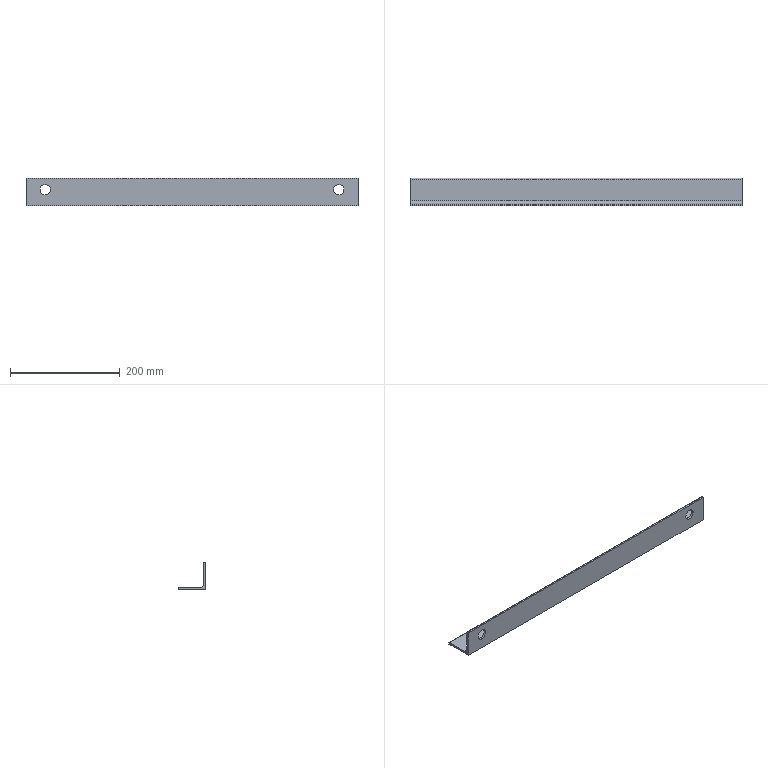Part | STEP file | 计量角钢1_Default<As Machined> | 1 solid | 15 faces | box 605 x 50 x 50 mm | volume 233520 mm3 | plane 8 | cylinder 7 | commonest cylinder face diameters 19 x4 2.66 x2 11 x1
STEP:
#1=CARTESIAN_POINT('',(0.,0.,0.));
#2=DIRECTION('',(0.,0.,1.));
#3=DIRECTION('',(1.,0.,0.));
#4=AXIS2_PLACEMENT_3D('',#1,#2,#3);
#5=CARTESIAN_POINT('',(-267.5,0.,38.585));
#6=VERTEX_POINT('',#5);
#7=CARTESIAN_POINT('',(-267.5,4.,38.585));
#8=VERTEX_POINT('',#7);
#9=CARTESIAN_POINT('',(-267.5,-6.,38.585));
#10=DIRECTION('',(0.,1.,0.));
#11=VECTOR('',#10,1.);
#12=LINE('',#9,#11);
#13=CARTESIAN_POINT('',(-267.5,-6.,29.085));
#14=DIRECTION('',(0.,1.,0.));
#15=DIRECTION('',(0.,0.,1.));
#16=AXIS2_PLACEMENT_3D('',#13,#14,#15);
#17=CYLINDRICAL_SURFACE('',#16,9.5);
#18=CARTESIAN_POINT('',(6.283,0.));
#19=DIRECTION('',(0.,1.));
#20=VECTOR('',#19,1.);
#21=LINE('',#18,#20);
#22=(GEOMETRIC_REPRESENTATION_CONTEXT(2)PARAMETRIC_REPRESENTATION_CONTEXT()REPRESENTATION_CONTEXT('',''));
#23=DEFINITIONAL_REPRESENTATION('',(#21),#22);
#24=PCURVE('',#17,#23);
#25=CARTESIAN_POINT('',(-267.5,-6.,29.085));
#26=DIRECTION('',(0.,1.,0.));
#27=DIRECTION('',(0.,0.,1.));
#28=AXIS2_PLACEMENT_3D('',#25,#26,#27);
#29=CYLINDRICAL_SURFACE('',#28,9.5);
#30=CARTESIAN_POINT('',(0.,0.));
#31=DIRECTION('',(0.,1.));
#32=VECTOR('',#31,1.);
#33=LINE('',#30,#32);
#34=(GEOMETRIC_REPRESENTATION_CONTEXT(2)PARAMETRIC_REPRESENTATION_CONTEXT()REPRESENTATION_CONTEXT('',''));
#35=DEFINITIONAL_REPRESENTATION('',(#33),#34);
#36=PCURVE('',#29,#35);
#37=SURFACE_CURVE('',#12,(#24,#36),.PCURVE_S1.);
#38=EDGE_CURVE('',#6,#8,#37,.T.);
#39=ORIENTED_EDGE('',*,*,#38,.T.);
#40=CARTESIAN_POINT('',(-267.5,4.,19.585));
#41=VERTEX_POINT('',#40);
#42=CARTESIAN_POINT('',(-267.5,4.,29.085));
#43=DIRECTION('',(0.,1.,0.));
#44=DIRECTION('',(0.,0.,1.));
#45=AXIS2_PLACEMENT_3D('',#42,#43,#44);
#46=CIRCLE('',#45,9.5);
#47=CARTESIAN_POINT('',(0.,10.));
#48=DIRECTION('',(1.,0.));
#49=VECTOR('',#48,1.);
#50=LINE('',#47,#49);
#51=(GEOMETRIC_REPRESENTATION_CONTEXT(2)PARAMETRIC_REPRESENTATION_CONTEXT()REPRESENTATION_CONTEXT('',''));
#52=DEFINITIONAL_REPRESENTATION('',(#50),#51);
#53=PCURVE('',#17,#52);
#54=CARTESIAN_POINT('',(302.5,4.,48.67));
#55=DIRECTION('',(0.,-1.,0.));
#56=DIRECTION('',(1.,0.,0.));
#57=AXIS2_PLACEMENT_3D('',#54,#55,#56);
#58=PLANE('',#57);
#59=CARTESIAN_POINT('',(-570.,-10.085));
#60=CARTESIAN_POINT('',(-553.546,-10.085));
#61=CARTESIAN_POINT('',(-561.773,-24.335));
#62=CARTESIAN_POINT('',(-570.,-38.585));
#63=CARTESIAN_POINT('',(-578.227,-24.335));
#64=CARTESIAN_POINT('',(-586.454,-10.085));
#65=CARTESIAN_POINT('',(-570.,-10.085));
#66=(BOUNDED_CURVE()B_SPLINE_CURVE(2,(#59,#60,#61,#62,#63,#64,#65),.UNSPECIFIED.,.T.,.F.)B_SPLINE_CURVE_WITH_KNOTS((1,2,2,2,2,1),(-2.094,0.,2.094,4.189,6.283,8.378),.UNSPECIFIED.)CURVE()GEOMETRIC_REPRESENTATION_ITEM()RATIONAL_B_SPLINE_CURVE((1.,0.5,1.,0.5,1.,0.5,1.))REPRESENTATION_ITEM(''));
#67=(GEOMETRIC_REPRESENTATION_CONTEXT(2)PARAMETRIC_REPRESENTATION_CONTEXT()REPRESENTATION_CONTEXT('',''));
#68=DEFINITIONAL_REPRESENTATION('',(#66),#67);
#69=PCURVE('',#58,#68);
#70=SURFACE_CURVE('',#46,(#53,#69),.PCURVE_S1.);
#71=EDGE_CURVE('',#41,#8,#70,.T.);
#72=ORIENTED_EDGE('',*,*,#71,.F.);
#73=CARTESIAN_POINT('',(-267.5,0.,19.585));
#74=VERTEX_POINT('',#73);
#75=CARTESIAN_POINT('',(-267.5,-6.,19.585));
#76=DIRECTION('',(0.,1.,0.));
#77=VECTOR('',#76,1.);
#78=LINE('',#75,#77);
#79=CARTESIAN_POINT('',(3.142,0.));
#80=DIRECTION('',(0.,1.));
#81=VECTOR('',#80,1.);
#82=LINE('',#79,#81);
#83=(GEOMETRIC_REPRESENTATION_CONTEXT(2)PARAMETRIC_REPRESENTATION_CONTEXT()REPRESENTATION_CONTEXT('',''));
#84=DEFINITIONAL_REPRESENTATION('',(#82),#83);
#85=PCURVE('',#17,#84);
#86=CARTESIAN_POINT('',(3.142,0.));
#87=DIRECTION('',(0.,1.));
#88=VECTOR('',#87,1.);
#89=LINE('',#86,#88);
#90=(GEOMETRIC_REPRESENTATION_CONTEXT(2)PARAMETRIC_REPRESENTATION_CONTEXT()REPRESENTATION_CONTEXT('',''));
#91=DEFINITIONAL_REPRESENTATION('',(#89),#90);
#92=PCURVE('',#29,#91);
#93=SURFACE_CURVE('',#78,(#85,#92),.PCURVE_S1.);
#94=EDGE_CURVE('',#74,#41,#93,.T.);
#95=ORIENTED_EDGE('',*,*,#94,.F.);
#96=CARTESIAN_POINT('',(-267.5,0.,29.085));
#97=DIRECTION('',(0.,1.,0.));
#98=DIRECTION('',(-1.,0.,0.));
#99=AXIS2_PLACEMENT_3D('',#96,#97,#98);
#100=CIRCLE('',#99,9.5);
#101=CARTESIAN_POINT('',(-1.571,6.));
#102=DIRECTION('',(1.,0.));
#103=VECTOR('',#102,1.);
#104=LINE('',#101,#103);
#105=(GEOMETRIC_REPRESENTATION_CONTEXT(2)PARAMETRIC_REPRESENTATION_CONTEXT()REPRESENTATION_CONTEXT('',''));
#106=DEFINITIONAL_REPRESENTATION('',(#104),#105);
#107=PCURVE('',#17,#106);
#108=CARTESIAN_POINT('',(302.5,0.,50.));
#109=DIRECTION('',(0.,1.,0.));
#110=DIRECTION('',(-1.,0.,0.));
#111=AXIS2_PLACEMENT_3D('',#108,#109,#110);
#112=PLANE('',#111);
#113=CARTESIAN_POINT('',(570.,-20.915));
#114=DIRECTION('',(1.,0.));
#115=AXIS2_PLACEMENT_2D('',#113,#114);
#116=CIRCLE('',#115,9.5);
#117=(GEOMETRIC_REPRESENTATION_CONTEXT(2)PARAMETRIC_REPRESENTATION_CONTEXT()REPRESENTATION_CONTEXT('',''));
#118=DEFINITIONAL_REPRESENTATION('',(#116),#117);
#119=PCURVE('',#112,#118);
#120=SURFACE_CURVE('',#100,(#107,#119),.PCURVE_S1.);
#121=EDGE_CURVE('',#74,#6,#120,.T.);
#122=ORIENTED_EDGE('',*,*,#121,.T.);
#123=EDGE_LOOP('',(#39,#72,#95,#122));
#124=FACE_BOUND('',#123,.F.);
#125=ADVANCED_FACE('',(#124),#17,.F.);
#126=CARTESIAN_POINT('',(267.5,0.,38.585));
#127=VERTEX_POINT('',#126);
#128=CARTESIAN_POINT('',(267.5,4.,38.585));
#129=VERTEX_POINT('',#128);
#130=CARTESIAN_POINT('',(267.5,-6.,38.585));
#131=DIRECTION('',(0.,1.,0.));
#132=VECTOR('',#131,1.);
#133=LINE('',#130,#132);
#134=CARTESIAN_POINT('',(267.5,-6.,29.085));
#135=DIRECTION('',(0.,1.,0.));
#136=DIRECTION('',(0.,0.,1.));
#137=AXIS2_PLACEMENT_3D('',#134,#135,#136);
#138=CYLINDRICAL_SURFACE('',#137,9.5);
#139=CARTESIAN_POINT('',(6.283,0.));
#140=DIRECTION('',(0.,1.));
#141=VECTOR('',#140,1.);
#142=LINE('',#139,#141);
#143=(GEOMETRIC_REPRESENTATION_CONTEXT(2)PARAMETRIC_REPRESENTATION_CONTEXT()REPRESENTATION_CONTEXT('',''));
#144=DEFINITIONAL_REPRESENTATION('',(#142),#143);
#145=PCURVE('',#138,#144);
#146=CARTESIAN_POINT('',(267.5,-6.,29.085));
#147=DIRECTION('',(0.,1.,0.));
#148=DIRECTION('',(0.,0.,1.));
#149=AXIS2_PLACEMENT_3D('',#146,#147,#148);
#150=CYLINDRICAL_SURFACE('',#149,9.5);
#151=CARTESIAN_POINT('',(0.,0.));
#152=DIRECTION('',(0.,1.));
#153=VECTOR('',#152,1.);
#154=LINE('',#151,#153);
#155=(GEOMETRIC_REPRESENTATION_CONTEXT(2)PARAMETRIC_REPRESENTATION_CONTEXT()REPRESENTATION_CONTEXT('',''));
#156=DEFINITIONAL_REPRESENTATION('',(#154),#155);
#157=PCURVE('',#150,#156);
#158=SURFACE_CURVE('',#133,(#145,#157),.PCURVE_S1.);
#159=EDGE_CURVE('',#127,#129,#158,.T.);
#160=ORIENTED_EDGE('',*,*,#159,.T.);
#161=CARTESIAN_POINT('',(267.5,4.,19.585));
#162=VERTEX_POINT('',#161);
#163=CARTESIAN_POINT('',(267.5,4.,29.085));
#164=DIRECTION('',(0.,1.,0.));
#165=DIRECTION('',(0.,0.,-1.));
#166=AXIS2_PLACEMENT_3D('',#163,#164,#165);
#167=CIRCLE('',#166,9.5);
#168=CARTESIAN_POINT('',(3.142,10.));
#169=DIRECTION('',(1.,0.));
#170=VECTOR('',#169,1.);
#171=LINE('',#168,#170);
#172=(GEOMETRIC_REPRESENTATION_CONTEXT(2)PARAMETRIC_REPRESENTATION_CONTEXT()REPRESENTATION_CONTEXT('',''));
#173=DEFINITIONAL_REPRESENTATION('',(#171),#172);
#174=PCURVE('',#138,#173);
#175=CARTESIAN_POINT('',(-35.,-29.085));
#176=CARTESIAN_POINT('',(-51.454,-29.085));
#177=CARTESIAN_POINT('',(-43.227,-14.835));
#178=CARTESIAN_POINT('',(-35.,-0.585));
#179=CARTESIAN_POINT('',(-26.773,-14.835));
#180=CARTESIAN_POINT('',(-18.546,-29.085));
#181=CARTESIAN_POINT('',(-35.,-29.085));
#182=(BOUNDED_CURVE()B_SPLINE_CURVE(2,(#175,#176,#177,#178,#179,#180,#181),.UNSPECIFIED.,.T.,.F.)B_SPLINE_CURVE_WITH_KNOTS((1,2,2,2,2,1),(-2.094,0.,2.094,4.189,6.283,8.378),.UNSPECIFIED.)CURVE()GEOMETRIC_REPRESENTATION_ITEM()RATIONAL_B_SPLINE_CURVE((1.,0.5,1.,0.5,1.,0.5,1.))REPRESENTATION_ITEM(''));
#183=(GEOMETRIC_REPRESENTATION_CONTEXT(2)PARAMETRIC_REPRESENTATION_CONTEXT()REPRESENTATION_CONTEXT('',''));
#184=DEFINITIONAL_REPRESENTATION('',(#182),#183);
#185=PCURVE('',#58,#184);
#186=SURFACE_CURVE('',#167,(#174,#185),.PCURVE_S1.);
#187=EDGE_CURVE('',#162,#129,#186,.T.);
#188=ORIENTED_EDGE('',*,*,#187,.F.);
#189=CARTESIAN_POINT('',(267.5,0.,19.585));
#190=VERTEX_POINT('',#189);
#191=CARTESIAN_POINT('',(267.5,-6.,19.585));
#192=DIRECTION('',(0.,1.,0.));
#193=VECTOR('',#192,1.);
#194=LINE('',#191,#193);
#195=CARTESIAN_POINT('',(3.142,0.));
#196=DIRECTION('',(0.,1.));
#197=VECTOR('',#196,1.);
#198=LINE('',#195,#197);
#199=(GEOMETRIC_REPRESENTATION_CONTEXT(2)PARAMETRIC_REPRESENTATION_CONTEXT()REPRESENTATION_CONTEXT('',''));
#200=DEFINITIONAL_REPRESENTATION('',(#198),#199);
#201=PCURVE('',#138,#200);
#202=CARTESIAN_POINT('',(3.142,0.));
#203=DIRECTION('',(0.,1.));
#204=VECTOR('',#203,1.);
#205=LINE('',#202,#204);
#206=(GEOMETRIC_REPRESENTATION_CONTEXT(2)PARAMETRIC_REPRESENTATION_CONTEXT()REPRESENTATION_CONTEXT('',''));
#207=DEFINITIONAL_REPRESENTATION('',(#205),#206);
#208=PCURVE('',#150,#207);
#209=SURFACE_CURVE('',#194,(#201,#208),.PCURVE_S1.);
#210=EDGE_CURVE('',#190,#162,#209,.T.);
#211=ORIENTED_EDGE('',*,*,#210,.F.);
#212=CARTESIAN_POINT('',(267.5,0.,29.085));
#213=DIRECTION('',(0.,1.,0.));
#214=DIRECTION('',(-1.,0.,0.));
#215=AXIS2_PLACEMENT_3D('',#212,#213,#214);
#216=CIRCLE('',#215,9.5);
#217=CARTESIAN_POINT('',(-1.571,6.));
#218=DIRECTION('',(1.,0.));
#219=VECTOR('',#218,1.);
#220=LINE('',#217,#219);
#221=(GEOMETRIC_REPRESENTATION_CONTEXT(2)PARAMETRIC_REPRESENTATION_CONTEXT()REPRESENTATION_CONTEXT('',''));
#222=DEFINITIONAL_REPRESENTATION('',(#220),#221);
#223=PCURVE('',#138,#222);
#224=CARTESIAN_POINT('',(35.,-20.915));
#225=DIRECTION('',(1.,0.));
#226=AXIS2_PLACEMENT_2D('',#224,#225);
#227=CIRCLE('',#226,9.5);
#228=(GEOMETRIC_REPRESENTATION_CONTEXT(2)PARAMETRIC_REPRESENTATION_CONTEXT()REPRESENTATION_CONTEXT('',''));
#229=DEFINITIONAL_REPRESENTATION('',(#227),#228);
#230=PCURVE('',#112,#229);
#231=SURFACE_CURVE('',#216,(#223,#230),.PCURVE_S1.);
#232=EDGE_CURVE('',#190,#127,#231,.T.);
#233=ORIENTED_EDGE('',*,*,#232,.T.);
#234=EDGE_LOOP('',(#160,#188,#211,#233));
#235=FACE_BOUND('',#234,.F.);
#236=ADVANCED_FACE('',(#235),#138,.F.);
#237=CARTESIAN_POINT('',(-302.5,50.,2.67));
#238=VERTEX_POINT('',#237);
#239=CARTESIAN_POINT('',(-302.5,48.67,4.));
#240=VERTEX_POINT('',#239);
#241=CARTESIAN_POINT('',(-302.5,48.67,2.67));
#242=DIRECTION('',(1.,0.,0.));
#243=DIRECTION('',(0.,1.,0.));
#244=AXIS2_PLACEMENT_3D('',#241,#242,#243);
#245=CIRCLE('',#244,1.33);
#246=CARTESIAN_POINT('',(302.5,48.67,2.67));
#247=DIRECTION('',(-1.,0.,0.));
#248=DIRECTION('',(0.,-1.,0.));
#249=AXIS2_PLACEMENT_3D('',#246,#247,#248);
#250=CYLINDRICAL_SURFACE('',#249,1.33);
#251=CARTESIAN_POINT('',(3.142,605.));
#252=DIRECTION('',(-1.,0.));
#253=VECTOR('',#252,1.);
#254=LINE('',#251,#253);
#255=(GEOMETRIC_REPRESENTATION_CONTEXT(2)PARAMETRIC_REPRESENTATION_CONTEXT()REPRESENTATION_CONTEXT('',''));
#256=DEFINITIONAL_REPRESENTATION('',(#254),#255);
#257=PCURVE('',#250,#256);
#258=CARTESIAN_POINT('',(-302.5,48.67,2.67));
#259=DIRECTION('',(1.,0.,0.));
#260=DIRECTION('',(0.,1.,0.));
#261=AXIS2_PLACEMENT_3D('',#258,#259,#260);
#262=PLANE('',#261);
#263=CARTESIAN_POINT('',(0.,0.));
#264=DIRECTION('',(1.,0.));
#265=AXIS2_PLACEMENT_2D('',#263,#264);
#266=CIRCLE('',#265,1.33);
#267=(GEOMETRIC_REPRESENTATION_CONTEXT(2)PARAMETRIC_REPRESENTATION_CONTEXT()REPRESENTATION_CONTEXT('',''));
#268=DEFINITIONAL_REPRESENTATION('',(#266),#267);
#269=PCURVE('',#262,#268);
#270=SURFACE_CURVE('',#245,(#257,#269),.PCURVE_S1.);
#271=EDGE_CURVE('',#238,#240,#270,.T.);
#272=ORIENTED_EDGE('',*,*,#271,.T.);
#273=CARTESIAN_POINT('',(302.5,48.67,4.));
#274=VERTEX_POINT('',#273);
#275=CARTESIAN_POINT('',(302.5,48.67,4.));
#276=DIRECTION('',(-1.,0.,0.));
#277=VECTOR('',#276,1.);
#278=LINE('',#275,#277);
#279=CARTESIAN_POINT('',(1.571,0.));
#280=DIRECTION('',(0.,1.));
#281=VECTOR('',#280,1.);
#282=LINE('',#279,#281);
#283=(GEOMETRIC_REPRESENTATION_CONTEXT(2)PARAMETRIC_REPRESENTATION_CONTEXT()REPRESENTATION_CONTEXT('',''));
#284=DEFINITIONAL_REPRESENTATION('',(#282),#283);
#285=PCURVE('',#250,#284);
#286=CARTESIAN_POINT('',(302.5,9.5,4.));
#287=DIRECTION('',(0.,0.,-1.));
#288=DIRECTION('',(-1.,0.,0.));
#289=AXIS2_PLACEMENT_3D('',#286,#287,#288);
#290=PLANE('',#289);
#291=CARTESIAN_POINT('',(0.,39.17));
#292=DIRECTION('',(1.,0.));
#293=VECTOR('',#292,1.);
#294=LINE('',#291,#293);
#295=(GEOMETRIC_REPRESENTATION_CONTEXT(2)PARAMETRIC_REPRESENTATION_CONTEXT()REPRESENTATION_CONTEXT('',''));
#296=DEFINITIONAL_REPRESENTATION('',(#294),#295);
#297=PCURVE('',#290,#296);
#298=SURFACE_CURVE('',#278,(#285,#297),.PCURVE_S1.);
#299=EDGE_CURVE('',#274,#240,#298,.T.);
#300=ORIENTED_EDGE('',*,*,#299,.F.);
#301=CARTESIAN_POINT('',(302.5,50.,2.67));
#302=VERTEX_POINT('',#301);
#303=CARTESIAN_POINT('',(302.5,48.67,2.67));
#304=DIRECTION('',(1.,0.,0.));
#305=DIRECTION('',(0.,1.,0.));
#306=AXIS2_PLACEMENT_3D('',#303,#304,#305);
#307=CIRCLE('',#306,1.33);
#308=CARTESIAN_POINT('',(3.142,0.));
#309=DIRECTION('',(-1.,0.));
#310=VECTOR('',#309,1.);
#311=LINE('',#308,#310);
#312=(GEOMETRIC_REPRESENTATION_CONTEXT(2)PARAMETRIC_REPRESENTATION_CONTEXT()REPRESENTATION_CONTEXT('',''));
#313=DEFINITIONAL_REPRESENTATION('',(#311),#312);
#314=PCURVE('',#250,#313);
#315=CARTESIAN_POINT('',(302.5,48.67,2.67));
#316=DIRECTION('',(1.,0.,0.));
#317=DIRECTION('',(0.,1.,0.));
#318=AXIS2_PLACEMENT_3D('',#315,#316,#317);
#319=PLANE('',#318);
#320=CARTESIAN_POINT('',(0.,0.));
#321=DIRECTION('',(1.,0.));
#322=AXIS2_PLACEMENT_2D('',#320,#321);
#323=CIRCLE('',#322,1.33);
#324=(GEOMETRIC_REPRESENTATION_CONTEXT(2)PARAMETRIC_REPRESENTATION_CONTEXT()REPRESENTATION_CONTEXT('',''));
#325=DEFINITIONAL_REPRESENTATION('',(#323),#324);
#326=PCURVE('',#319,#325);
#327=SURFACE_CURVE('',#307,(#314,#326),.PCURVE_S1.);
#328=EDGE_CURVE('',#302,#274,#327,.T.);
#329=ORIENTED_EDGE('',*,*,#328,.F.);
#330=CARTESIAN_POINT('',(302.5,50.,2.67));
#331=DIRECTION('',(-1.,0.,0.));
#332=VECTOR('',#331,1.);
#333=LINE('',#330,#332);
#334=CARTESIAN_POINT('',(3.142,0.));
#335=DIRECTION('',(0.,1.));
#336=VECTOR('',#335,1.);
#337=LINE('',#334,#336);
#338=(GEOMETRIC_REPRESENTATION_CONTEXT(2)PARAMETRIC_REPRESENTATION_CONTEXT()REPRESENTATION_CONTEXT('',''));
#339=DEFINITIONAL_REPRESENTATION('',(#337),#338);
#340=PCURVE('',#250,#339);
#341=CARTESIAN_POINT('',(302.5,50.,2.67));
#342=DIRECTION('',(0.,-1.,0.));
#343=DIRECTION('',(1.,0.,0.));
#344=AXIS2_PLACEMENT_3D('',#341,#342,#343);
#345=PLANE('',#344);
#346=CARTESIAN_POINT('',(0.,0.));
#347=DIRECTION('',(-1.,0.));
#348=VECTOR('',#347,1.);
#349=LINE('',#346,#348);
#350=(GEOMETRIC_REPRESENTATION_CONTEXT(2)PARAMETRIC_REPRESENTATION_CONTEXT()REPRESENTATION_CONTEXT('',''));
#351=DEFINITIONAL_REPRESENTATION('',(#349),#350);
#352=PCURVE('',#345,#351);
#353=SURFACE_CURVE('',#333,(#340,#352),.PCURVE_S1.);
#354=EDGE_CURVE('',#302,#238,#353,.T.);
#355=ORIENTED_EDGE('',*,*,#354,.T.);
#356=EDGE_LOOP('',(#272,#300,#329,#355));
#357=FACE_BOUND('',#356,.T.);
#358=ADVANCED_FACE('',(#357),#250,.T.);
#359=CARTESIAN_POINT('',(-302.5,9.5,4.));
#360=VERTEX_POINT('',#359);
#361=CARTESIAN_POINT('',(-302.5,9.5,4.));
#362=DIRECTION('',(0.,-1.,0.));
#363=VECTOR('',#362,1.);
#364=LINE('',#361,#363);
#365=CARTESIAN_POINT('',(605.,0.));
#366=DIRECTION('',(0.,-1.));
#367=VECTOR('',#366,1.);
#368=LINE('',#365,#367);
#369=(GEOMETRIC_REPRESENTATION_CONTEXT(2)PARAMETRIC_REPRESENTATION_CONTEXT()REPRESENTATION_CONTEXT('',''));
#370=DEFINITIONAL_REPRESENTATION('',(#368),#369);
#371=PCURVE('',#290,#370);
#372=CARTESIAN_POINT('',(-39.17,1.33));
#373=DIRECTION('',(-1.,0.));
#374=VECTOR('',#373,1.);
#375=LINE('',#372,#374);
#376=(GEOMETRIC_REPRESENTATION_CONTEXT(2)PARAMETRIC_REPRESENTATION_CONTEXT()REPRESENTATION_CONTEXT('',''));
#377=DEFINITIONAL_REPRESENTATION('',(#375),#376);
#378=PCURVE('',#262,#377);
#379=SURFACE_CURVE('',#364,(#371,#378),.PCURVE_S1.);
#380=EDGE_CURVE('',#240,#360,#379,.T.);
#381=ORIENTED_EDGE('',*,*,#380,.T.);
#382=CARTESIAN_POINT('',(302.5,9.5,4.));
#383=VERTEX_POINT('',#382);
#384=CARTESIAN_POINT('',(302.5,9.5,4.));
#385=DIRECTION('',(-1.,0.,0.));
#386=VECTOR('',#385,1.);
#387=LINE('',#384,#386);
#388=CARTESIAN_POINT('',(0.,0.));
#389=DIRECTION('',(1.,0.));
#390=VECTOR('',#389,1.);
#391=LINE('',#388,#390);
#392=(GEOMETRIC_REPRESENTATION_CONTEXT(2)PARAMETRIC_REPRESENTATION_CONTEXT()REPRESENTATION_CONTEXT('',''));
#393=DEFINITIONAL_REPRESENTATION('',(#391),#392);
#394=PCURVE('',#290,#393);
#395=CARTESIAN_POINT('',(302.5,9.5,9.5));
#396=DIRECTION('',(-1.,0.,0.));
#397=DIRECTION('',(0.,-1.,0.));
#398=AXIS2_PLACEMENT_3D('',#395,#396,#397);
#399=CYLINDRICAL_SURFACE('',#398,5.5);
#400=CARTESIAN_POINT('',(4.712,0.));
#401=DIRECTION('',(0.,1.));
#402=VECTOR('',#401,1.);
#403=LINE('',#400,#402);
#404=(GEOMETRIC_REPRESENTATION_CONTEXT(2)PARAMETRIC_REPRESENTATION_CONTEXT()REPRESENTATION_CONTEXT('',''));
#405=DEFINITIONAL_REPRESENTATION('',(#403),#404);
#406=PCURVE('',#399,#405);
#407=SURFACE_CURVE('',#387,(#394,#406),.PCURVE_S1.);
#408=EDGE_CURVE('',#383,#360,#407,.T.);
#409=ORIENTED_EDGE('',*,*,#408,.F.);
#410=CARTESIAN_POINT('',(302.5,9.5,4.));
#411=DIRECTION('',(0.,-1.,0.));
#412=VECTOR('',#411,1.);
#413=LINE('',#410,#412);
#414=CARTESIAN_POINT('',(0.,0.));
#415=DIRECTION('',(0.,-1.));
#416=VECTOR('',#415,1.);
#417=LINE('',#414,#416);
#418=(GEOMETRIC_REPRESENTATION_CONTEXT(2)PARAMETRIC_REPRESENTATION_CONTEXT()REPRESENTATION_CONTEXT('',''));
#419=DEFINITIONAL_REPRESENTATION('',(#417),#418);
#420=PCURVE('',#290,#419);
#421=CARTESIAN_POINT('',(-39.17,1.33));
#422=DIRECTION('',(-1.,0.));
#423=VECTOR('',#422,1.);
#424=LINE('',#421,#423);
#425=(GEOMETRIC_REPRESENTATION_CONTEXT(2)PARAMETRIC_REPRESENTATION_CONTEXT()REPRESENTATION_CONTEXT('',''));
#426=DEFINITIONAL_REPRESENTATION('',(#424),#425);
#427=PCURVE('',#319,#426);
#428=SURFACE_CURVE('',#413,(#420,#427),.PCURVE_S1.);
#429=EDGE_CURVE('',#274,#383,#428,.T.);
#430=ORIENTED_EDGE('',*,*,#429,.F.);
#431=ORIENTED_EDGE('',*,*,#299,.T.);
#432=EDGE_LOOP('',(#381,#409,#430,#431));
#433=FACE_BOUND('',#432,.T.);
#434=ADVANCED_FACE('',(#433),#290,.F.);
#435=ORIENTED_EDGE('',*,*,#408,.F.);
#436=CARTESIAN_POINT('',(302.5,4.,9.5));
#437=VERTEX_POINT('',#436);
#438=CARTESIAN_POINT('',(302.5,9.5,9.5));
#439=DIRECTION('',(-1.,0.,0.));
#440=DIRECTION('',(0.,1.,0.));
#441=AXIS2_PLACEMENT_3D('',#438,#439,#440);
#442=CIRCLE('',#441,5.5);
#443=CARTESIAN_POINT('',(3.142,0.));
#444=DIRECTION('',(1.,0.));
#445=VECTOR('',#444,1.);
#446=LINE('',#443,#445);
#447=(GEOMETRIC_REPRESENTATION_CONTEXT(2)PARAMETRIC_REPRESENTATION_CONTEXT()REPRESENTATION_CONTEXT('',''));
#448=DEFINITIONAL_REPRESENTATION('',(#446),#447);
#449=PCURVE('',#399,#448);
#450=CARTESIAN_POINT('',(-33.67,6.83));
#451=CARTESIAN_POINT('',(-33.67,-2.696));
#452=CARTESIAN_POINT('',(-41.92,2.067));
#453=CARTESIAN_POINT('',(-50.17,6.83));
#454=CARTESIAN_POINT('',(-41.92,11.593));
#455=CARTESIAN_POINT('',(-33.67,16.356));
#456=CARTESIAN_POINT('',(-33.67,6.83));
#457=(BOUNDED_CURVE()B_SPLINE_CURVE(2,(#450,#451,#452,#453,#454,#455,#456),.UNSPECIFIED.,.T.,.F.)B_SPLINE_CURVE_WITH_KNOTS((1,2,2,2,2,1),(-2.094,0.,2.094,4.189,6.283,8.378),.UNSPECIFIED.)CURVE()GEOMETRIC_REPRESENTATION_ITEM()RATIONAL_B_SPLINE_CURVE((1.,0.5,1.,0.5,1.,0.5,1.))REPRESENTATION_ITEM(''));
#458=(GEOMETRIC_REPRESENTATION_CONTEXT(2)PARAMETRIC_REPRESENTATION_CONTEXT()REPRESENTATION_CONTEXT('',''));
#459=DEFINITIONAL_REPRESENTATION('',(#457),#458);
#460=PCURVE('',#319,#459);
#461=SURFACE_CURVE('',#442,(#449,#460),.PCURVE_S1.);
#462=EDGE_CURVE('',#383,#437,#461,.T.);
#463=ORIENTED_EDGE('',*,*,#462,.T.);
#464=CARTESIAN_POINT('',(-302.5,4.,9.5));
#465=VERTEX_POINT('',#464);
#466=CARTESIAN_POINT('',(302.5,4.,9.5));
#467=DIRECTION('',(-1.,0.,0.));
#468=VECTOR('',#467,1.);
#469=LINE('',#466,#468);
#470=CARTESIAN_POINT('',(6.283,0.));
#471=DIRECTION('',(0.,1.));
#472=VECTOR('',#471,1.);
#473=LINE('',#470,#472);
#474=(GEOMETRIC_REPRESENTATION_CONTEXT(2)PARAMETRIC_REPRESENTATION_CONTEXT()REPRESENTATION_CONTEXT('',''));
#475=DEFINITIONAL_REPRESENTATION('',(#473),#474);
#476=PCURVE('',#399,#475);
#477=CARTESIAN_POINT('',(0.,-39.17));
#478=DIRECTION('',(-1.,0.));
#479=VECTOR('',#478,1.);
#480=LINE('',#477,#479);
#481=(GEOMETRIC_REPRESENTATION_CONTEXT(2)PARAMETRIC_REPRESENTATION_CONTEXT()REPRESENTATION_CONTEXT('',''));
#482=DEFINITIONAL_REPRESENTATION('',(#480),#481);
#483=PCURVE('',#58,#482);
#484=SURFACE_CURVE('',#469,(#476,#483),.PCURVE_S1.);
#485=EDGE_CURVE('',#437,#465,#484,.T.);
#486=ORIENTED_EDGE('',*,*,#485,.T.);
#487=CARTESIAN_POINT('',(-302.5,9.5,9.5));
#488=DIRECTION('',(-1.,0.,0.));
#489=DIRECTION('',(0.,1.,0.));
#490=AXIS2_PLACEMENT_3D('',#487,#488,#489);
#491=CIRCLE('',#490,5.5);
#492=CARTESIAN_POINT('',(3.142,605.));
#493=DIRECTION('',(1.,0.));
#494=VECTOR('',#493,1.);
#495=LINE('',#492,#494);
#496=(GEOMETRIC_REPRESENTATION_CONTEXT(2)PARAMETRIC_REPRESENTATION_CONTEXT()REPRESENTATION_CONTEXT('',''));
#497=DEFINITIONAL_REPRESENTATION('',(#495),#496);
#498=PCURVE('',#399,#497);
#499=CARTESIAN_POINT('',(-33.67,6.83));
#500=CARTESIAN_POINT('',(-33.67,-2.696));
#501=CARTESIAN_POINT('',(-41.92,2.067));
#502=CARTESIAN_POINT('',(-50.17,6.83));
#503=CARTESIAN_POINT('',(-41.92,11.593));
#504=CARTESIAN_POINT('',(-33.67,16.356));
#505=CARTESIAN_POINT('',(-33.67,6.83));
#506=(BOUNDED_CURVE()B_SPLINE_CURVE(2,(#499,#500,#501,#502,#503,#504,#505),.UNSPECIFIED.,.T.,.F.)B_SPLINE_CURVE_WITH_KNOTS((1,2,2,2,2,1),(-2.094,0.,2.094,4.189,6.283,8.378),.UNSPECIFIED.)CURVE()GEOMETRIC_REPRESENTATION_ITEM()RATIONAL_B_SPLINE_CURVE((1.,0.5,1.,0.5,1.,0.5,1.))REPRESENTATION_ITEM(''));
#507=(GEOMETRIC_REPRESENTATION_CONTEXT(2)PARAMETRIC_REPRESENTATION_CONTEXT()REPRESENTATION_CONTEXT('',''));
#508=DEFINITIONAL_REPRESENTATION('',(#506),#507);
#509=PCURVE('',#262,#508);
#510=SURFACE_CURVE('',#491,(#498,#509),.PCURVE_S1.);
#511=EDGE_CURVE('',#360,#465,#510,.T.);
#512=ORIENTED_EDGE('',*,*,#511,.F.);
#513=EDGE_LOOP('',(#435,#463,#486,#512));
#514=FACE_BOUND('',#513,.F.);
#515=ADVANCED_FACE('',(#514),#399,.F.);
#516=CARTESIAN_POINT('',(-267.5,4.,29.085));
#517=DIRECTION('',(0.,1.,0.));
#518=DIRECTION('',(0.,0.,1.));
#519=AXIS2_PLACEMENT_3D('',#516,#517,#518);
#520=CIRCLE('',#519,9.5);
#521=CARTESIAN_POINT('',(-570.,-10.085));
#522=CARTESIAN_POINT('',(-553.546,-10.085));
#523=CARTESIAN_POINT('',(-561.773,-24.335));
#524=CARTESIAN_POINT('',(-570.,-38.585));
#525=CARTESIAN_POINT('',(-578.227,-24.335));
#526=CARTESIAN_POINT('',(-586.454,-10.085));
#527=CARTESIAN_POINT('',(-570.,-10.085));
#528=(BOUNDED_CURVE()B_SPLINE_CURVE(2,(#521,#522,#523,#524,#525,#526,#527),.UNSPECIFIED.,.T.,.F.)B_SPLINE_CURVE_WITH_KNOTS((1,2,2,2,2,1),(-2.094,0.,2.094,4.189,6.283,8.378),.UNSPECIFIED.)CURVE()GEOMETRIC_REPRESENTATION_ITEM()RATIONAL_B_SPLINE_CURVE((1.,0.5,1.,0.5,1.,0.5,1.))REPRESENTATION_ITEM(''));
#529=(GEOMETRIC_REPRESENTATION_CONTEXT(2)PARAMETRIC_REPRESENTATION_CONTEXT()REPRESENTATION_CONTEXT('',''));
#530=DEFINITIONAL_REPRESENTATION('',(#528),#529);
#531=PCURVE('',#58,#530);
#532=CARTESIAN_POINT('',(0.,10.));
#533=DIRECTION('',(1.,0.));
#534=VECTOR('',#533,1.);
#535=LINE('',#532,#534);
#536=(GEOMETRIC_REPRESENTATION_CONTEXT(2)PARAMETRIC_REPRESENTATION_CONTEXT()REPRESENTATION_CONTEXT('',''));
#537=DEFINITIONAL_REPRESENTATION('',(#535),#536);
#538=PCURVE('',#29,#537);
#539=SURFACE_CURVE('',#520,(#531,#538),.PCURVE_S1.);
#540=EDGE_CURVE('',#8,#41,#539,.T.);
#541=ORIENTED_EDGE('',*,*,#540,.F.);
#542=ORIENTED_EDGE('',*,*,#71,.F.);
#543=EDGE_LOOP('',(#541,#542));
#544=FACE_BOUND('',#543,.T.);
#545=CARTESIAN_POINT('',(267.5,4.,29.085));
#546=DIRECTION('',(0.,1.,0.));
#547=DIRECTION('',(0.,0.,-1.));
#548=AXIS2_PLACEMENT_3D('',#545,#546,#547);
#549=CIRCLE('',#548,9.5);
#550=CARTESIAN_POINT('',(-35.,-29.085));
#551=CARTESIAN_POINT('',(-51.454,-29.085));
#552=CARTESIAN_POINT('',(-43.227,-14.835));
#553=CARTESIAN_POINT('',(-35.,-0.585));
#554=CARTESIAN_POINT('',(-26.773,-14.835));
#555=CARTESIAN_POINT('',(-18.546,-29.085));
#556=CARTESIAN_POINT('',(-35.,-29.085));
#557=(BOUNDED_CURVE()B_SPLINE_CURVE(2,(#550,#551,#552,#553,#554,#555,#556),.UNSPECIFIED.,.T.,.F.)B_SPLINE_CURVE_WITH_KNOTS((1,2,2,2,2,1),(-2.094,0.,2.094,4.189,6.283,8.378),.UNSPECIFIED.)CURVE()GEOMETRIC_REPRESENTATION_ITEM()RATIONAL_B_SPLINE_CURVE((1.,0.5,1.,0.5,1.,0.5,1.))REPRESENTATION_ITEM(''));
#558=(GEOMETRIC_REPRESENTATION_CONTEXT(2)PARAMETRIC_REPRESENTATION_CONTEXT()REPRESENTATION_CONTEXT('',''));
#559=DEFINITIONAL_REPRESENTATION('',(#557),#558);
#560=PCURVE('',#58,#559);
#561=CARTESIAN_POINT('',(-3.142,10.));
#562=DIRECTION('',(1.,0.));
#563=VECTOR('',#562,1.);
#564=LINE('',#561,#563);
#565=(GEOMETRIC_REPRESENTATION_CONTEXT(2)PARAMETRIC_REPRESENTATION_CONTEXT()REPRESENTATION_CONTEXT('',''));
#566=DEFINITIONAL_REPRESENTATION('',(#564),#565);
#567=PCURVE('',#150,#566);
#568=SURFACE_CURVE('',#549,(#560,#567),.PCURVE_S1.);
#569=EDGE_CURVE('',#129,#162,#568,.T.);
#570=ORIENTED_EDGE('',*,*,#569,.F.);
#571=ORIENTED_EDGE('',*,*,#187,.F.);
#572=EDGE_LOOP('',(#570,#571));
#573=FACE_BOUND('',#572,.T.);
#574=CARTESIAN_POINT('',(-302.5,4.,48.67));
#575=VERTEX_POINT('',#574);
#576=CARTESIAN_POINT('',(-302.5,4.,48.67));
#577=DIRECTION('',(0.,0.,1.));
#578=VECTOR('',#577,1.);
#579=LINE('',#576,#578);
#580=CARTESIAN_POINT('',(-605.,0.));
#581=DIRECTION('',(0.,1.));
#582=VECTOR('',#581,1.);
#583=LINE('',#580,#582);
#584=(GEOMETRIC_REPRESENTATION_CONTEXT(2)PARAMETRIC_REPRESENTATION_CONTEXT()REPRESENTATION_CONTEXT('',''));
#585=DEFINITIONAL_REPRESENTATION('',(#583),#584);
#586=PCURVE('',#58,#585);
#587=CARTESIAN_POINT('',(-44.67,46.));
#588=DIRECTION('',(0.,1.));
#589=VECTOR('',#588,1.);
#590=LINE('',#587,#589);
#591=(GEOMETRIC_REPRESENTATION_CONTEXT(2)PARAMETRIC_REPRESENTATION_CONTEXT()REPRESENTATION_CONTEXT('',''));
#592=DEFINITIONAL_REPRESENTATION('',(#590),#591);
#593=PCURVE('',#262,#592);
#594=SURFACE_CURVE('',#579,(#586,#593),.PCURVE_S1.);
#595=EDGE_CURVE('',#465,#575,#594,.T.);
#596=ORIENTED_EDGE('',*,*,#595,.T.);
#597=CARTESIAN_POINT('',(302.5,4.,48.67));
#598=VERTEX_POINT('',#597);
#599=CARTESIAN_POINT('',(302.5,4.,48.67));
#600=DIRECTION('',(-1.,0.,0.));
#601=VECTOR('',#600,1.);
#602=LINE('',#599,#601);
#603=CARTESIAN_POINT('',(0.,0.));
#604=DIRECTION('',(-1.,0.));
#605=VECTOR('',#604,1.);
#606=LINE('',#603,#605);
#607=(GEOMETRIC_REPRESENTATION_CONTEXT(2)PARAMETRIC_REPRESENTATION_CONTEXT()REPRESENTATION_CONTEXT('',''));
#608=DEFINITIONAL_REPRESENTATION('',(#606),#607);
#609=PCURVE('',#58,#608);
#610=CARTESIAN_POINT('',(302.5,2.67,48.67));
#611=DIRECTION('',(-1.,0.,0.));
#612=DIRECTION('',(0.,-1.,0.));
#613=AXIS2_PLACEMENT_3D('',#610,#611,#612);
#614=CYLINDRICAL_SURFACE('',#613,1.33);
#615=CARTESIAN_POINT('',(3.142,0.));
#616=DIRECTION('',(0.,1.));
#617=VECTOR('',#616,1.);
#618=LINE('',#615,#617);
#619=(GEOMETRIC_REPRESENTATION_CONTEXT(2)PARAMETRIC_REPRESENTATION_CONTEXT()REPRESENTATION_CONTEXT('',''));
#620=DEFINITIONAL_REPRESENTATION('',(#618),#619);
#621=PCURVE('',#614,#620);
#622=SURFACE_CURVE('',#602,(#609,#621),.PCURVE_S1.);
#623=EDGE_CURVE('',#598,#575,#622,.T.);
#624=ORIENTED_EDGE('',*,*,#623,.F.);
#625=CARTESIAN_POINT('',(302.5,4.,48.67));
#626=DIRECTION('',(0.,0.,1.));
#627=VECTOR('',#626,1.);
#628=LINE('',#625,#627);
#629=CARTESIAN_POINT('',(0.,0.));
#630=DIRECTION('',(0.,1.));
#631=VECTOR('',#630,1.);
#632=LINE('',#629,#631);
#633=(GEOMETRIC_REPRESENTATION_CONTEXT(2)PARAMETRIC_REPRESENTATION_CONTEXT()REPRESENTATION_CONTEXT('',''));
#634=DEFINITIONAL_REPRESENTATION('',(#632),#633);
#635=PCURVE('',#58,#634);
#636=CARTESIAN_POINT('',(-44.67,46.));
#637=DIRECTION('',(0.,1.));
#638=VECTOR('',#637,1.);
#639=LINE('',#636,#638);
#640=(GEOMETRIC_REPRESENTATION_CONTEXT(2)PARAMETRIC_REPRESENTATION_CONTEXT()REPRESENTATION_CONTEXT('',''));
#641=DEFINITIONAL_REPRESENTATION('',(#639),#640);
#642=PCURVE('',#319,#641);
#643=SURFACE_CURVE('',#628,(#635,#642),.PCURVE_S1.);
#644=EDGE_CURVE('',#437,#598,#643,.T.);
#645=ORIENTED_EDGE('',*,*,#644,.F.);
#646=ORIENTED_EDGE('',*,*,#485,.T.);
#647=EDGE_LOOP('',(#596,#624,#645,#646));
#648=FACE_BOUND('',#647,.T.);
#649=ADVANCED_FACE('',(#544,#573,#648),#58,.F.);
#650=CARTESIAN_POINT('',(-302.5,2.67,50.));
#651=VERTEX_POINT('',#650);
#652=CARTESIAN_POINT('',(-302.5,2.67,48.67));
#653=DIRECTION('',(1.,0.,0.));
#654=DIRECTION('',(0.,1.,0.));
#655=AXIS2_PLACEMENT_3D('',#652,#653,#654);
#656=CIRCLE('',#655,1.33);
#657=CARTESIAN_POINT('',(3.142,605.));
#658=DIRECTION('',(-1.,0.));
#659=VECTOR('',#658,1.);
#660=LINE('',#657,#659);
#661=(GEOMETRIC_REPRESENTATION_CONTEXT(2)PARAMETRIC_REPRESENTATION_CONTEXT()REPRESENTATION_CONTEXT('',''));
#662=DEFINITIONAL_REPRESENTATION('',(#660),#661);
#663=PCURVE('',#614,#662);
#664=CARTESIAN_POINT('',(-46.,46.));
#665=DIRECTION('',(1.,0.));
#666=AXIS2_PLACEMENT_2D('',#664,#665);
#667=CIRCLE('',#666,1.33);
#668=(GEOMETRIC_REPRESENTATION_CONTEXT(2)PARAMETRIC_REPRESENTATION_CONTEXT()REPRESENTATION_CONTEXT('',''));
#669=DEFINITIONAL_REPRESENTATION('',(#667),#668);
#670=PCURVE('',#262,#669);
#671=SURFACE_CURVE('',#656,(#663,#670),.PCURVE_S1.);
#672=EDGE_CURVE('',#575,#651,#671,.T.);
#673=ORIENTED_EDGE('',*,*,#672,.T.);
#674=CARTESIAN_POINT('',(302.5,2.67,50.));
#675=VERTEX_POINT('',#674);
#676=CARTESIAN_POINT('',(302.5,2.67,50.));
#677=DIRECTION('',(-1.,0.,0.));
#678=VECTOR('',#677,1.);
#679=LINE('',#676,#678);
#680=CARTESIAN_POINT('',(1.571,0.));
#681=DIRECTION('',(0.,1.));
#682=VECTOR('',#681,1.);
#683=LINE('',#680,#682);
#684=(GEOMETRIC_REPRESENTATION_CONTEXT(2)PARAMETRIC_REPRESENTATION_CONTEXT()REPRESENTATION_CONTEXT('',''));
#685=DEFINITIONAL_REPRESENTATION('',(#683),#684);
#686=PCURVE('',#614,#685);
#687=CARTESIAN_POINT('',(302.5,0.,50.));
#688=DIRECTION('',(0.,0.,-1.));
#689=DIRECTION('',(0.,1.,0.));
#690=AXIS2_PLACEMENT_3D('',#687,#688,#689);
#691=PLANE('',#690);
#692=CARTESIAN_POINT('',(2.67,0.));
#693=DIRECTION('',(0.,-1.));
#694=VECTOR('',#693,1.);
#695=LINE('',#692,#694);
#696=(GEOMETRIC_REPRESENTATION_CONTEXT(2)PARAMETRIC_REPRESENTATION_CONTEXT()REPRESENTATION_CONTEXT('',''));
#697=DEFINITIONAL_REPRESENTATION('',(#695),#696);
#698=PCURVE('',#691,#697);
#699=SURFACE_CURVE('',#679,(#686,#698),.PCURVE_S1.);
#700=EDGE_CURVE('',#675,#651,#699,.T.);
#701=ORIENTED_EDGE('',*,*,#700,.F.);
#702=CARTESIAN_POINT('',(302.5,2.67,48.67));
#703=DIRECTION('',(1.,0.,0.));
#704=DIRECTION('',(0.,1.,0.));
#705=AXIS2_PLACEMENT_3D('',#702,#703,#704);
#706=CIRCLE('',#705,1.33);
#707=CARTESIAN_POINT('',(3.142,0.));
#708=DIRECTION('',(-1.,0.));
#709=VECTOR('',#708,1.);
#710=LINE('',#707,#709);
#711=(GEOMETRIC_REPRESENTATION_CONTEXT(2)PARAMETRIC_REPRESENTATION_CONTEXT()REPRESENTATION_CONTEXT('',''));
#712=DEFINITIONAL_REPRESENTATION('',(#710),#711);
#713=PCURVE('',#614,#712);
#714=CARTESIAN_POINT('',(-46.,46.));
#715=DIRECTION('',(1.,0.));
#716=AXIS2_PLACEMENT_2D('',#714,#715);
#717=CIRCLE('',#716,1.33);
#718=(GEOMETRIC_REPRESENTATION_CONTEXT(2)PARAMETRIC_REPRESENTATION_CONTEXT()REPRESENTATION_CONTEXT('',''));
#719=DEFINITIONAL_REPRESENTATION('',(#717),#718);
#720=PCURVE('',#319,#719);
#721=SURFACE_CURVE('',#706,(#713,#720),.PCURVE_S1.);
#722=EDGE_CURVE('',#598,#675,#721,.T.);
#723=ORIENTED_EDGE('',*,*,#722,.F.);
#724=ORIENTED_EDGE('',*,*,#623,.T.);
#725=EDGE_LOOP('',(#673,#701,#723,#724));
#726=FACE_BOUND('',#725,.T.);
#727=ADVANCED_FACE('',(#726),#614,.T.);
#728=CARTESIAN_POINT('',(-302.5,0.,50.));
#729=VERTEX_POINT('',#728);
#730=CARTESIAN_POINT('',(-302.5,0.,50.));
#731=DIRECTION('',(0.,-1.,0.));
#732=VECTOR('',#731,1.);
#733=LINE('',#730,#732);
#734=CARTESIAN_POINT('',(0.,-605.));
#735=DIRECTION('',(-1.,0.));
#736=VECTOR('',#735,1.);
#737=LINE('',#734,#736);
#738=(GEOMETRIC_REPRESENTATION_CONTEXT(2)PARAMETRIC_REPRESENTATION_CONTEXT()REPRESENTATION_CONTEXT('',''));
#739=DEFINITIONAL_REPRESENTATION('',(#737),#738);
#740=PCURVE('',#691,#739);
#741=CARTESIAN_POINT('',(-48.67,47.33));
#742=DIRECTION('',(-1.,0.));
#743=VECTOR('',#742,1.);
#744=LINE('',#741,#743);
#745=(GEOMETRIC_REPRESENTATION_CONTEXT(2)PARAMETRIC_REPRESENTATION_CONTEXT()REPRESENTATION_CONTEXT('',''));
#746=DEFINITIONAL_REPRESENTATION('',(#744),#745);
#747=PCURVE('',#262,#746);
#748=SURFACE_CURVE('',#733,(#740,#747),.PCURVE_S1.);
#749=EDGE_CURVE('',#651,#729,#748,.T.);
#750=ORIENTED_EDGE('',*,*,#749,.T.);
#751=CARTESIAN_POINT('',(302.5,0.,50.));
#752=VERTEX_POINT('',#751);
#753=CARTESIAN_POINT('',(302.5,0.,50.));
#754=DIRECTION('',(-1.,0.,0.));
#755=VECTOR('',#754,1.);
#756=LINE('',#753,#755);
#757=CARTESIAN_POINT('',(0.,0.));
#758=DIRECTION('',(0.,-1.));
#759=VECTOR('',#758,1.);
#760=LINE('',#757,#759);
#761=(GEOMETRIC_REPRESENTATION_CONTEXT(2)PARAMETRIC_REPRESENTATION_CONTEXT()REPRESENTATION_CONTEXT('',''));
#762=DEFINITIONAL_REPRESENTATION('',(#760),#761);
#763=PCURVE('',#691,#762);
#764=CARTESIAN_POINT('',(0.,0.));
#765=DIRECTION('',(1.,0.));
#766=VECTOR('',#765,1.);
#767=LINE('',#764,#766);
#768=(GEOMETRIC_REPRESENTATION_CONTEXT(2)PARAMETRIC_REPRESENTATION_CONTEXT()REPRESENTATION_CONTEXT('',''));
#769=DEFINITIONAL_REPRESENTATION('',(#767),#768);
#770=PCURVE('',#112,#769);
#771=SURFACE_CURVE('',#756,(#763,#770),.PCURVE_S1.);
#772=EDGE_CURVE('',#752,#729,#771,.T.);
#773=ORIENTED_EDGE('',*,*,#772,.F.);
#774=CARTESIAN_POINT('',(302.5,0.,50.));
#775=DIRECTION('',(0.,-1.,0.));
#776=VECTOR('',#775,1.);
#777=LINE('',#774,#776);
#778=CARTESIAN_POINT('',(0.,0.));
#779=DIRECTION('',(-1.,0.));
#780=VECTOR('',#779,1.);
#781=LINE('',#778,#780);
#782=(GEOMETRIC_REPRESENTATION_CONTEXT(2)PARAMETRIC_REPRESENTATION_CONTEXT()REPRESENTATION_CONTEXT('',''));
#783=DEFINITIONAL_REPRESENTATION('',(#781),#782);
#784=PCURVE('',#691,#783);
#785=CARTESIAN_POINT('',(-48.67,47.33));
#786=DIRECTION('',(-1.,0.));
#787=VECTOR('',#786,1.);
#788=LINE('',#785,#787);
#789=(GEOMETRIC_REPRESENTATION_CONTEXT(2)PARAMETRIC_REPRESENTATION_CONTEXT()REPRESENTATION_CONTEXT('',''));
#790=DEFINITIONAL_REPRESENTATION('',(#788),#789);
#791=PCURVE('',#319,#790);
#792=SURFACE_CURVE('',#777,(#784,#791),.PCURVE_S1.);
#793=EDGE_CURVE('',#675,#752,#792,.T.);
#794=ORIENTED_EDGE('',*,*,#793,.F.);
#795=ORIENTED_EDGE('',*,*,#700,.T.);
#796=EDGE_LOOP('',(#750,#773,#794,#795));
#797=FACE_BOUND('',#796,.T.);
#798=ADVANCED_FACE('',(#797),#691,.F.);
#799=CARTESIAN_POINT('',(-267.5,0.,29.085));
#800=DIRECTION('',(0.,1.,0.));
#801=DIRECTION('',(-1.,0.,0.));
#802=AXIS2_PLACEMENT_3D('',#799,#800,#801);
#803=CIRCLE('',#802,9.5);
#804=CARTESIAN_POINT('',(570.,-20.915));
#805=DIRECTION('',(1.,0.));
#806=AXIS2_PLACEMENT_2D('',#804,#805);
#807=CIRCLE('',#806,9.5);
#808=(GEOMETRIC_REPRESENTATION_CONTEXT(2)PARAMETRIC_REPRESENTATION_CONTEXT()REPRESENTATION_CONTEXT('',''));
#809=DEFINITIONAL_REPRESENTATION('',(#807),#808);
#810=PCURVE('',#112,#809);
#811=CARTESIAN_POINT('',(-1.571,6.));
#812=DIRECTION('',(1.,0.));
#813=VECTOR('',#812,1.);
#814=LINE('',#811,#813);
#815=(GEOMETRIC_REPRESENTATION_CONTEXT(2)PARAMETRIC_REPRESENTATION_CONTEXT()REPRESENTATION_CONTEXT('',''));
#816=DEFINITIONAL_REPRESENTATION('',(#814),#815);
#817=PCURVE('',#29,#816);
#818=SURFACE_CURVE('',#803,(#810,#817),.PCURVE_S1.);
#819=EDGE_CURVE('',#6,#74,#818,.T.);
#820=ORIENTED_EDGE('',*,*,#819,.T.);
#821=ORIENTED_EDGE('',*,*,#121,.T.);
#822=EDGE_LOOP('',(#820,#821));
#823=FACE_BOUND('',#822,.T.);
#824=CARTESIAN_POINT('',(267.5,0.,29.085));
#825=DIRECTION('',(0.,1.,0.));
#826=DIRECTION('',(-1.,0.,0.));
#827=AXIS2_PLACEMENT_3D('',#824,#825,#826);
#828=CIRCLE('',#827,9.5);
#829=CARTESIAN_POINT('',(35.,-20.915));
#830=DIRECTION('',(1.,0.));
#831=AXIS2_PLACEMENT_2D('',#829,#830);
#832=CIRCLE('',#831,9.5);
#833=(GEOMETRIC_REPRESENTATION_CONTEXT(2)PARAMETRIC_REPRESENTATION_CONTEXT()REPRESENTATION_CONTEXT('',''));
#834=DEFINITIONAL_REPRESENTATION('',(#832),#833);
#835=PCURVE('',#112,#834);
#836=CARTESIAN_POINT('',(-1.571,6.));
#837=DIRECTION('',(1.,0.));
#838=VECTOR('',#837,1.);
#839=LINE('',#836,#838);
#840=(GEOMETRIC_REPRESENTATION_CONTEXT(2)PARAMETRIC_REPRESENTATION_CONTEXT()REPRESENTATION_CONTEXT('',''));
#841=DEFINITIONAL_REPRESENTATION('',(#839),#840);
#842=PCURVE('',#150,#841);
#843=SURFACE_CURVE('',#828,(#835,#842),.PCURVE_S1.);
#844=EDGE_CURVE('',#127,#190,#843,.T.);
#845=ORIENTED_EDGE('',*,*,#844,.T.);
#846=ORIENTED_EDGE('',*,*,#232,.T.);
#847=EDGE_LOOP('',(#845,#846));
#848=FACE_BOUND('',#847,.T.);
#849=CARTESIAN_POINT('',(-302.5,0.,0.));
#850=VERTEX_POINT('',#849);
#851=CARTESIAN_POINT('',(-302.5,0.,50.));
#852=DIRECTION('',(0.,0.,-1.));
#853=VECTOR('',#852,1.);
#854=LINE('',#851,#853);
#855=CARTESIAN_POINT('',(605.,0.));
#856=DIRECTION('',(0.,-1.));
#857=VECTOR('',#856,1.);
#858=LINE('',#855,#857);
#859=(GEOMETRIC_REPRESENTATION_CONTEXT(2)PARAMETRIC_REPRESENTATION_CONTEXT()REPRESENTATION_CONTEXT('',''));
#860=DEFINITIONAL_REPRESENTATION('',(#858),#859);
#861=PCURVE('',#112,#860);
#862=CARTESIAN_POINT('',(-48.67,47.33));
#863=DIRECTION('',(0.,-1.));
#864=VECTOR('',#863,1.);
#865=LINE('',#862,#864);
#866=(GEOMETRIC_REPRESENTATION_CONTEXT(2)PARAMETRIC_REPRESENTATION_CONTEXT()REPRESENTATION_CONTEXT('',''));
#867=DEFINITIONAL_REPRESENTATION('',(#865),#866);
#868=PCURVE('',#262,#867);
#869=SURFACE_CURVE('',#854,(#861,#868),.PCURVE_S1.);
#870=EDGE_CURVE('',#729,#850,#869,.T.);
#871=ORIENTED_EDGE('',*,*,#870,.T.);
#872=CARTESIAN_POINT('',(302.5,0.,0.));
#873=VERTEX_POINT('',#872);
#874=CARTESIAN_POINT('',(302.5,0.,0.));
#875=DIRECTION('',(-1.,0.,0.));
#876=VECTOR('',#875,1.);
#877=LINE('',#874,#876);
#878=CARTESIAN_POINT('',(0.,-50.));
#879=DIRECTION('',(1.,0.));
#880=VECTOR('',#879,1.);
#881=LINE('',#878,#880);
#882=(GEOMETRIC_REPRESENTATION_CONTEXT(2)PARAMETRIC_REPRESENTATION_CONTEXT()REPRESENTATION_CONTEXT('',''));
#883=DEFINITIONAL_REPRESENTATION('',(#881),#882);
#884=PCURVE('',#112,#883);
#885=CARTESIAN_POINT('',(302.5,0.,0.));
#886=DIRECTION('',(0.,0.,1.));
#887=DIRECTION('',(1.,0.,0.));
#888=AXIS2_PLACEMENT_3D('',#885,#886,#887);
#889=PLANE('',#888);
#890=CARTESIAN_POINT('',(0.,0.));
#891=DIRECTION('',(-1.,0.));
#892=VECTOR('',#891,1.);
#893=LINE('',#890,#892);
#894=(GEOMETRIC_REPRESENTATION_CONTEXT(2)PARAMETRIC_REPRESENTATION_CONTEXT()REPRESENTATION_CONTEXT('',''));
#895=DEFINITIONAL_REPRESENTATION('',(#893),#894);
#896=PCURVE('',#889,#895);
#897=SURFACE_CURVE('',#877,(#884,#896),.PCURVE_S1.);
#898=EDGE_CURVE('',#873,#850,#897,.T.);
#899=ORIENTED_EDGE('',*,*,#898,.F.);
#900=CARTESIAN_POINT('',(302.5,0.,50.));
#901=DIRECTION('',(0.,0.,-1.));
#902=VECTOR('',#901,1.);
#903=LINE('',#900,#902);
#904=CARTESIAN_POINT('',(0.,0.));
#905=DIRECTION('',(0.,-1.));
#906=VECTOR('',#905,1.);
#907=LINE('',#904,#906);
#908=(GEOMETRIC_REPRESENTATION_CONTEXT(2)PARAMETRIC_REPRESENTATION_CONTEXT()REPRESENTATION_CONTEXT('',''));
#909=DEFINITIONAL_REPRESENTATION('',(#907),#908);
#910=PCURVE('',#112,#909);
#911=CARTESIAN_POINT('',(-48.67,47.33));
#912=DIRECTION('',(0.,-1.));
#913=VECTOR('',#912,1.);
#914=LINE('',#911,#913);
#915=(GEOMETRIC_REPRESENTATION_CONTEXT(2)PARAMETRIC_REPRESENTATION_CONTEXT()REPRESENTATION_CONTEXT('',''));
#916=DEFINITIONAL_REPRESENTATION('',(#914),#915);
#917=PCURVE('',#319,#916);
#918=SURFACE_CURVE('',#903,(#910,#917),.PCURVE_S1.);
#919=EDGE_CURVE('',#752,#873,#918,.T.);
#920=ORIENTED_EDGE('',*,*,#919,.F.);
#921=ORIENTED_EDGE('',*,*,#772,.T.);
#922=EDGE_LOOP('',(#871,#899,#920,#921));
#923=FACE_BOUND('',#922,.T.);
#924=ADVANCED_FACE('',(#823,#848,#923),#112,.F.);
#925=CARTESIAN_POINT('',(-302.5,50.,0.));
#926=VERTEX_POINT('',#925);
#927=CARTESIAN_POINT('',(-302.5,0.,0.));
#928=DIRECTION('',(0.,1.,0.));
#929=VECTOR('',#928,1.);
#930=LINE('',#927,#929);
#931=CARTESIAN_POINT('',(-605.,0.));
#932=DIRECTION('',(0.,1.));
#933=VECTOR('',#932,1.);
#934=LINE('',#931,#933);
#935=(GEOMETRIC_REPRESENTATION_CONTEXT(2)PARAMETRIC_REPRESENTATION_CONTEXT()REPRESENTATION_CONTEXT('',''));
#936=DEFINITIONAL_REPRESENTATION('',(#934),#935);
#937=PCURVE('',#889,#936);
#938=CARTESIAN_POINT('',(-48.67,-2.67));
#939=DIRECTION('',(1.,0.));
#940=VECTOR('',#939,1.);
#941=LINE('',#938,#940);
#942=(GEOMETRIC_REPRESENTATION_CONTEXT(2)PARAMETRIC_REPRESENTATION_CONTEXT()REPRESENTATION_CONTEXT('',''));
#943=DEFINITIONAL_REPRESENTATION('',(#941),#942);
#944=PCURVE('',#262,#943);
#945=SURFACE_CURVE('',#930,(#937,#944),.PCURVE_S1.);
#946=EDGE_CURVE('',#850,#926,#945,.T.);
#947=ORIENTED_EDGE('',*,*,#946,.T.);
#948=CARTESIAN_POINT('',(302.5,50.,0.));
#949=VERTEX_POINT('',#948);
#950=CARTESIAN_POINT('',(302.5,50.,0.));
#951=DIRECTION('',(-1.,0.,0.));
#952=VECTOR('',#951,1.);
#953=LINE('',#950,#952);
#954=CARTESIAN_POINT('',(0.,50.));
#955=DIRECTION('',(-1.,0.));
#956=VECTOR('',#955,1.);
#957=LINE('',#954,#956);
#958=(GEOMETRIC_REPRESENTATION_CONTEXT(2)PARAMETRIC_REPRESENTATION_CONTEXT()REPRESENTATION_CONTEXT('',''));
#959=DEFINITIONAL_REPRESENTATION('',(#957),#958);
#960=PCURVE('',#889,#959);
#961=CARTESIAN_POINT('',(0.,-2.67));
#962=DIRECTION('',(-1.,0.));
#963=VECTOR('',#962,1.);
#964=LINE('',#961,#963);
#965=(GEOMETRIC_REPRESENTATION_CONTEXT(2)PARAMETRIC_REPRESENTATION_CONTEXT()REPRESENTATION_CONTEXT('',''));
#966=DEFINITIONAL_REPRESENTATION('',(#964),#965);
#967=PCURVE('',#345,#966);
#968=SURFACE_CURVE('',#953,(#960,#967),.PCURVE_S1.);
#969=EDGE_CURVE('',#949,#926,#968,.T.);
#970=ORIENTED_EDGE('',*,*,#969,.F.);
#971=CARTESIAN_POINT('',(302.5,0.,0.));
#972=DIRECTION('',(0.,1.,0.));
#973=VECTOR('',#972,1.);
#974=LINE('',#971,#973);
#975=CARTESIAN_POINT('',(0.,0.));
#976=DIRECTION('',(0.,1.));
#977=VECTOR('',#976,1.);
#978=LINE('',#975,#977);
#979=(GEOMETRIC_REPRESENTATION_CONTEXT(2)PARAMETRIC_REPRESENTATION_CONTEXT()REPRESENTATION_CONTEXT('',''));
#980=DEFINITIONAL_REPRESENTATION('',(#978),#979);
#981=PCURVE('',#889,#980);
#982=CARTESIAN_POINT('',(-48.67,-2.67));
#983=DIRECTION('',(1.,0.));
#984=VECTOR('',#983,1.);
#985=LINE('',#982,#984);
#986=(GEOMETRIC_REPRESENTATION_CONTEXT(2)PARAMETRIC_REPRESENTATION_CONTEXT()REPRESENTATION_CONTEXT('',''));
#987=DEFINITIONAL_REPRESENTATION('',(#985),#986);
#988=PCURVE('',#319,#987);
#989=SURFACE_CURVE('',#974,(#981,#988),.PCURVE_S1.);
#990=EDGE_CURVE('',#873,#949,#989,.T.);
#991=ORIENTED_EDGE('',*,*,#990,.F.);
#992=ORIENTED_EDGE('',*,*,#898,.T.);
#993=EDGE_LOOP('',(#947,#970,#991,#992));
#994=FACE_BOUND('',#993,.T.);
#995=ADVANCED_FACE('',(#994),#889,.F.);
#996=CARTESIAN_POINT('',(-302.5,50.,2.67));
#997=DIRECTION('',(0.,0.,1.));
#998=VECTOR('',#997,1.);
#999=LINE('',#996,#998);
#1000=CARTESIAN_POINT('',(-605.,0.));
#1001=DIRECTION('',(0.,1.));
#1002=VECTOR('',#1001,1.);
#1003=LINE('',#1000,#1002);
#1004=(GEOMETRIC_REPRESENTATION_CONTEXT(2)PARAMETRIC_REPRESENTATION_CONTEXT()REPRESENTATION_CONTEXT('',''));
#1005=DEFINITIONAL_REPRESENTATION('',(#1003),#1004);
#1006=PCURVE('',#345,#1005);
#1007=CARTESIAN_POINT('',(1.33,0.));
#1008=DIRECTION('',(0.,1.));
#1009=VECTOR('',#1008,1.);
#1010=LINE('',#1007,#1009);
#1011=(GEOMETRIC_REPRESENTATION_CONTEXT(2)PARAMETRIC_REPRESENTATION_CONTEXT()REPRESENTATION_CONTEXT('',''));
#1012=DEFINITIONAL_REPRESENTATION('',(#1010),#1011);
#1013=PCURVE('',#262,#1012);
#1014=SURFACE_CURVE('',#999,(#1006,#1013),.PCURVE_S1.);
#1015=EDGE_CURVE('',#926,#238,#1014,.T.);
#1016=ORIENTED_EDGE('',*,*,#1015,.T.);
#1017=ORIENTED_EDGE('',*,*,#354,.F.);
#1018=CARTESIAN_POINT('',(302.5,50.,2.67));
#1019=DIRECTION('',(0.,0.,1.));
#1020=VECTOR('',#1019,1.);
#1021=LINE('',#1018,#1020);
#1022=CARTESIAN_POINT('',(0.,0.));
#1023=DIRECTION('',(0.,1.));
#1024=VECTOR('',#1023,1.);
#1025=LINE('',#1022,#1024);
#1026=(GEOMETRIC_REPRESENTATION_CONTEXT(2)PARAMETRIC_REPRESENTATION_CONTEXT()REPRESENTATION_CONTEXT('',''));
#1027=DEFINITIONAL_REPRESENTATION('',(#1025),#1026);
#1028=PCURVE('',#345,#1027);
#1029=CARTESIAN_POINT('',(1.33,0.));
#1030=DIRECTION('',(0.,1.));
#1031=VECTOR('',#1030,1.);
#1032=LINE('',#1029,#1031);
#1033=(GEOMETRIC_REPRESENTATION_CONTEXT(2)PARAMETRIC_REPRESENTATION_CONTEXT()REPRESENTATION_CONTEXT('',''));
#1034=DEFINITIONAL_REPRESENTATION('',(#1032),#1033);
#1035=PCURVE('',#319,#1034);
#1036=SURFACE_CURVE('',#1021,(#1028,#1035),.PCURVE_S1.);
#1037=EDGE_CURVE('',#949,#302,#1036,.T.);
#1038=ORIENTED_EDGE('',*,*,#1037,.F.);
#1039=ORIENTED_EDGE('',*,*,#969,.T.);
#1040=EDGE_LOOP('',(#1016,#1017,#1038,#1039));
#1041=FACE_BOUND('',#1040,.T.);
#1042=ADVANCED_FACE('',(#1041),#345,.F.);
#1043=ORIENTED_EDGE('',*,*,#328,.T.);
#1044=ORIENTED_EDGE('',*,*,#429,.T.);
#1045=ORIENTED_EDGE('',*,*,#462,.T.);
#1046=ORIENTED_EDGE('',*,*,#644,.T.);
#1047=ORIENTED_EDGE('',*,*,#722,.T.);
#1048=ORIENTED_EDGE('',*,*,#793,.T.);
#1049=ORIENTED_EDGE('',*,*,#919,.T.);
#1050=ORIENTED_EDGE('',*,*,#990,.T.);
#1051=ORIENTED_EDGE('',*,*,#1037,.T.);
#1052=EDGE_LOOP('',(#1043,#1044,#1045,#1046,#1047,#1048,#1049,#1050,#1051));
#1053=FACE_BOUND('',#1052,.T.);
#1054=ADVANCED_FACE('',(#1053),#319,.T.);
#1055=ORIENTED_EDGE('',*,*,#271,.F.);
#1056=ORIENTED_EDGE('',*,*,#1015,.F.);
#1057=ORIENTED_EDGE('',*,*,#946,.F.);
#1058=ORIENTED_EDGE('',*,*,#870,.F.);
#1059=ORIENTED_EDGE('',*,*,#749,.F.);
#1060=ORIENTED_EDGE('',*,*,#672,.F.);
#1061=ORIENTED_EDGE('',*,*,#595,.F.);
#1062=ORIENTED_EDGE('',*,*,#511,.F.);
#1063=ORIENTED_EDGE('',*,*,#380,.F.);
#1064=EDGE_LOOP('',(#1055,#1056,#1057,#1058,#1059,#1060,#1061,#1062,#1063));
#1065=FACE_BOUND('',#1064,.T.);
#1066=ADVANCED_FACE('',(#1065),#262,.F.);
#1067=ORIENTED_EDGE('',*,*,#569,.F.);
#1068=ORIENTED_EDGE('',*,*,#159,.F.);
#1069=ORIENTED_EDGE('',*,*,#844,.T.);
#1070=ORIENTED_EDGE('',*,*,#210,.T.);
#1071=EDGE_LOOP('',(#1067,#1068,#1069,#1070));
#1072=FACE_BOUND('',#1071,.F.);
#1073=ADVANCED_FACE('',(#1072),#150,.F.);
#1074=ORIENTED_EDGE('',*,*,#540,.F.);
#1075=ORIENTED_EDGE('',*,*,#38,.F.);
#1076=ORIENTED_EDGE('',*,*,#819,.T.);
#1077=ORIENTED_EDGE('',*,*,#94,.T.);
#1078=EDGE_LOOP('',(#1074,#1075,#1076,#1077));
#1079=FACE_BOUND('',#1078,.F.);
#1080=ADVANCED_FACE('',(#1079),#29,.F.);
#1081=CLOSED_SHELL('',(#125,#236,#358,#434,#515,#649,#727,#798,#924,#995,#1042,#1054,#1066,#1073,#1080));
#1082=MANIFOLD_SOLID_BREP('',#1081);
#1083=(LENGTH_UNIT()NAMED_UNIT(*)SI_UNIT(.MILLI.,.METRE.));
#1084=UNCERTAINTY_MEASURE_WITH_UNIT(LENGTH_MEASURE(0.0000001),#1083,'','');
#1085=(NAMED_UNIT(*)PLANE_ANGLE_UNIT()SI_UNIT($,.RADIAN.));
#1086=(NAMED_UNIT(*)SI_UNIT($,.STERADIAN.)SOLID_ANGLE_UNIT());
#1087=(GEOMETRIC_REPRESENTATION_CONTEXT(3)GLOBAL_UNCERTAINTY_ASSIGNED_CONTEXT((#1084))GLOBAL_UNIT_ASSIGNED_CONTEXT((#1083,#1085,#1086))REPRESENTATION_CONTEXT('',''));
#1088=ADVANCED_BREP_SHAPE_REPRESENTATION('',(#4,#1082),#1087);